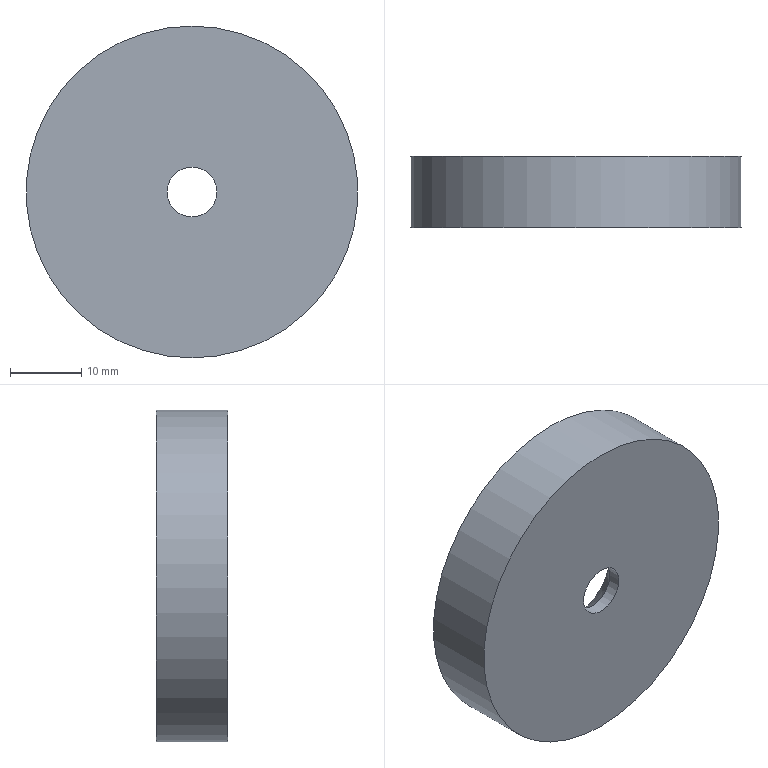Part | STEP file | Lower part of clamping device | 1 solid | 11 faces | box 46.5 x 10 x 46.5 mm | volume 11861 mm3 | plane 5 | cone 3 | cylinder 3 | commonest cylinder face diameters 7 x1 22 x1 46.5 x1
STEP:
#1=CARTESIAN_POINT('',(0.,0.,23.25));
#2=VERTEX_POINT('',#1);
#3=CARTESIAN_POINT('',(0.,0.,0.));
#4=DIRECTION('',(0.,1.,0.));
#5=DIRECTION('',(0.,0.,1.));
#6=AXIS2_PLACEMENT_3D('',#3,#4,#5);
#7=CIRCLE('',#6,23.25);
#8=EDGE_CURVE('',#2,#2,#7,.T.);
#9=ORIENTED_EDGE('',*,*,#8,.F.);
#10=EDGE_LOOP('',(#9));
#11=FACE_BOUND('',#10,.T.);
#12=CARTESIAN_POINT('',(3.5,0.,0.));
#13=VERTEX_POINT('',#12);
#14=CARTESIAN_POINT('',(0.,0.,0.));
#15=DIRECTION('',(0.,1.,0.));
#16=DIRECTION('',(1.,0.,0.));
#17=AXIS2_PLACEMENT_3D('',#14,#15,#16);
#18=CIRCLE('',#17,3.5);
#19=EDGE_CURVE('',#13,#13,#18,.T.);
#20=ORIENTED_EDGE('',*,*,#19,.T.);
#21=EDGE_LOOP('',(#20));
#22=FACE_BOUND('',#21,.T.);
#23=CARTESIAN_POINT('',(0.,0.,0.));
#24=DIRECTION('',(0.,-1.,0.));
#25=DIRECTION('',(0.,0.,1.));
#26=AXIS2_PLACEMENT_3D('',#23,#24,#25);
#27=PLANE('',#26);
#28=ADVANCED_FACE('',(#11,#22),#27,.T.);
#29=CARTESIAN_POINT('',(0.,5.,11.));
#30=VERTEX_POINT('',#29);
#31=CARTESIAN_POINT('',(0.,5.,0.));
#32=DIRECTION('',(0.,1.,0.));
#33=DIRECTION('',(0.,0.,1.));
#34=AXIS2_PLACEMENT_3D('',#31,#32,#33);
#35=CIRCLE('',#34,11.);
#36=EDGE_CURVE('',#30,#30,#35,.T.);
#37=ORIENTED_EDGE('',*,*,#36,.T.);
#38=EDGE_LOOP('',(#37));
#39=FACE_BOUND('',#38,.T.);
#40=CARTESIAN_POINT('',(6.72,5.,0.));
#41=VERTEX_POINT('',#40);
#42=CARTESIAN_POINT('',(0.,5.,0.));
#43=DIRECTION('',(0.,1.,0.));
#44=DIRECTION('',(1.,0.,0.));
#45=AXIS2_PLACEMENT_3D('',#42,#43,#44);
#46=CIRCLE('',#45,6.72);
#47=EDGE_CURVE('',#41,#41,#46,.F.);
#48=ORIENTED_EDGE('',*,*,#47,.T.);
#49=EDGE_LOOP('',(#48));
#50=FACE_BOUND('',#49,.T.);
#51=CARTESIAN_POINT('',(0.,5.,0.));
#52=DIRECTION('',(0.,1.,0.));
#53=DIRECTION('',(0.,0.,1.));
#54=AXIS2_PLACEMENT_3D('',#51,#52,#53);
#55=PLANE('',#54);
#56=ADVANCED_FACE('',(#39,#50),#55,.T.);
#57=ORIENTED_EDGE('',*,*,#47,.F.);
#58=EDGE_LOOP('',(#57));
#59=FACE_OUTER_BOUND('',#58,.T.);
#60=CARTESIAN_POINT('',(3.5,1.78,0.));
#61=VERTEX_POINT('',#60);
#62=CARTESIAN_POINT('',(0.,1.78,0.));
#63=DIRECTION('',(0.,1.,0.));
#64=DIRECTION('',(1.,0.,0.));
#65=AXIS2_PLACEMENT_3D('',#62,#63,#64);
#66=CIRCLE('',#65,3.5);
#67=EDGE_CURVE('',#61,#61,#66,.T.);
#68=ORIENTED_EDGE('',*,*,#67,.F.);
#69=EDGE_LOOP('',(#68));
#70=FACE_OUTER_BOUND('',#69,.T.);
#71=CARTESIAN_POINT('',(0.,3.39,0.));
#72=DIRECTION('',(0.,1.,0.));
#73=DIRECTION('',(1.,0.,0.));
#74=AXIS2_PLACEMENT_3D('',#71,#72,#73);
#75=CONICAL_SURFACE('',#74,5.11,0.7854);
#76=ADVANCED_FACE('',(#59,#70),#75,.F.);
#77=ORIENTED_EDGE('',*,*,#67,.T.);
#78=EDGE_LOOP('',(#77));
#79=FACE_OUTER_BOUND('',#78,.T.);
#80=ORIENTED_EDGE('',*,*,#19,.F.);
#81=EDGE_LOOP('',(#80));
#82=FACE_OUTER_BOUND('',#81,.T.);
#83=CARTESIAN_POINT('',(0.,-35.,0.));
#84=DIRECTION('',(0.,1.,0.));
#85=DIRECTION('',(1.,0.,0.));
#86=AXIS2_PLACEMENT_3D('',#83,#84,#85);
#87=CYLINDRICAL_SURFACE('',#86,3.5);
#88=ADVANCED_FACE('',(#79,#82),#87,.F.);
#89=CARTESIAN_POINT('',(0.,10.,23.25));
#90=VERTEX_POINT('',#89);
#91=CARTESIAN_POINT('',(0.,10.,0.));
#92=DIRECTION('',(0.,1.,0.));
#93=DIRECTION('',(0.,0.,1.));
#94=AXIS2_PLACEMENT_3D('',#91,#92,#93);
#95=CIRCLE('',#94,23.25);
#96=EDGE_CURVE('',#90,#90,#95,.T.);
#97=ORIENTED_EDGE('',*,*,#96,.F.);
#98=EDGE_LOOP('',(#97));
#99=FACE_OUTER_BOUND('',#98,.T.);
#100=ORIENTED_EDGE('',*,*,#8,.T.);
#101=EDGE_LOOP('',(#100));
#102=FACE_OUTER_BOUND('',#101,.T.);
#103=CARTESIAN_POINT('',(0.,0.,0.));
#104=DIRECTION('',(0.,1.,0.));
#105=DIRECTION('',(0.,0.,1.));
#106=AXIS2_PLACEMENT_3D('',#103,#104,#105);
#107=CYLINDRICAL_SURFACE('',#106,23.25);
#108=ADVANCED_FACE('',(#99,#102),#107,.T.);
#109=CARTESIAN_POINT('',(0.,7.5,11.));
#110=VERTEX_POINT('',#109);
#111=CARTESIAN_POINT('',(0.,7.5,0.));
#112=DIRECTION('',(0.,1.,0.));
#113=DIRECTION('',(0.,0.,1.));
#114=AXIS2_PLACEMENT_3D('',#111,#112,#113);
#115=CIRCLE('',#114,11.);
#116=EDGE_CURVE('',#110,#110,#115,.T.);
#117=ORIENTED_EDGE('',*,*,#116,.T.);
#118=EDGE_LOOP('',(#117));
#119=FACE_OUTER_BOUND('',#118,.T.);
#120=ORIENTED_EDGE('',*,*,#36,.F.);
#121=EDGE_LOOP('',(#120));
#122=FACE_OUTER_BOUND('',#121,.T.);
#123=CARTESIAN_POINT('',(0.,7.5,0.));
#124=DIRECTION('',(0.,1.,0.));
#125=DIRECTION('',(0.,0.,1.));
#126=AXIS2_PLACEMENT_3D('',#123,#124,#125);
#127=CYLINDRICAL_SURFACE('',#126,11.);
#128=ADVANCED_FACE('',(#119,#122),#127,.F.);
#129=ORIENTED_EDGE('',*,*,#96,.T.);
#130=EDGE_LOOP('',(#129));
#131=FACE_BOUND('',#130,.T.);
#132=CARTESIAN_POINT('',(0.,10.,22.25));
#133=VERTEX_POINT('',#132);
#134=CARTESIAN_POINT('',(0.,10.,0.));
#135=DIRECTION('',(0.,1.,0.));
#136=DIRECTION('',(0.,0.,1.));
#137=AXIS2_PLACEMENT_3D('',#134,#135,#136);
#138=CIRCLE('',#137,22.25);
#139=EDGE_CURVE('',#133,#133,#138,.T.);
#140=ORIENTED_EDGE('',*,*,#139,.F.);
#141=EDGE_LOOP('',(#140));
#142=FACE_BOUND('',#141,.T.);
#143=CARTESIAN_POINT('',(0.,10.,0.));
#144=DIRECTION('',(0.,1.,0.));
#145=DIRECTION('',(0.,0.,1.));
#146=AXIS2_PLACEMENT_3D('',#143,#144,#145);
#147=PLANE('',#146);
#148=ADVANCED_FACE('',(#131,#142),#147,.T.);
#149=CARTESIAN_POINT('',(0.,7.5,12.));
#150=VERTEX_POINT('',#149);
#151=CARTESIAN_POINT('',(0.,7.5,0.));
#152=DIRECTION('',(0.,1.,0.));
#153=DIRECTION('',(0.,0.,1.));
#154=AXIS2_PLACEMENT_3D('',#151,#152,#153);
#155=CIRCLE('',#154,12.);
#156=EDGE_CURVE('',#150,#150,#155,.T.);
#157=ORIENTED_EDGE('',*,*,#156,.T.);
#158=EDGE_LOOP('',(#157));
#159=FACE_BOUND('',#158,.T.);
#160=ORIENTED_EDGE('',*,*,#116,.F.);
#161=EDGE_LOOP('',(#160));
#162=FACE_BOUND('',#161,.T.);
#163=CARTESIAN_POINT('',(0.,7.5,0.));
#164=DIRECTION('',(0.,1.,0.));
#165=DIRECTION('',(0.,0.,1.));
#166=AXIS2_PLACEMENT_3D('',#163,#164,#165);
#167=PLANE('',#166);
#168=ADVANCED_FACE('',(#159,#162),#167,.T.);
#169=ORIENTED_EDGE('',*,*,#139,.T.);
#170=EDGE_LOOP('',(#169));
#171=FACE_OUTER_BOUND('',#170,.T.);
#172=CARTESIAN_POINT('',(0.,7.,19.25));
#173=VERTEX_POINT('',#172);
#174=CARTESIAN_POINT('',(0.,7.,0.));
#175=DIRECTION('',(0.,1.,0.));
#176=DIRECTION('',(0.,0.,1.));
#177=AXIS2_PLACEMENT_3D('',#174,#175,#176);
#178=CIRCLE('',#177,19.25);
#179=EDGE_CURVE('',#173,#173,#178,.T.);
#180=ORIENTED_EDGE('',*,*,#179,.F.);
#181=EDGE_LOOP('',(#180));
#182=FACE_OUTER_BOUND('',#181,.T.);
#183=CARTESIAN_POINT('',(0.,8.5,0.));
#184=DIRECTION('',(0.,1.,0.));
#185=DIRECTION('',(0.,0.,1.));
#186=AXIS2_PLACEMENT_3D('',#183,#184,#185);
#187=CONICAL_SURFACE('',#186,20.75,0.7854);
#188=ADVANCED_FACE('',(#171,#182),#187,.F.);
#189=ORIENTED_EDGE('',*,*,#156,.F.);
#190=EDGE_LOOP('',(#189));
#191=FACE_OUTER_BOUND('',#190,.T.);
#192=CARTESIAN_POINT('',(0.,7.,12.5));
#193=VERTEX_POINT('',#192);
#194=CARTESIAN_POINT('',(0.,7.,0.));
#195=DIRECTION('',(0.,1.,0.));
#196=DIRECTION('',(0.,0.,1.));
#197=AXIS2_PLACEMENT_3D('',#194,#195,#196);
#198=CIRCLE('',#197,12.5);
#199=EDGE_CURVE('',#193,#193,#198,.T.);
#200=ORIENTED_EDGE('',*,*,#199,.T.);
#201=EDGE_LOOP('',(#200));
#202=FACE_OUTER_BOUND('',#201,.T.);
#203=CARTESIAN_POINT('',(0.,7.25,0.));
#204=DIRECTION('',(0.,-1.,0.));
#205=DIRECTION('',(0.,0.,-1.));
#206=AXIS2_PLACEMENT_3D('',#203,#204,#205);
#207=CONICAL_SURFACE('',#206,12.25,0.7854);
#208=ADVANCED_FACE('',(#191,#202),#207,.T.);
#209=ORIENTED_EDGE('',*,*,#179,.T.);
#210=EDGE_LOOP('',(#209));
#211=FACE_BOUND('',#210,.T.);
#212=ORIENTED_EDGE('',*,*,#199,.F.);
#213=EDGE_LOOP('',(#212));
#214=FACE_BOUND('',#213,.T.);
#215=CARTESIAN_POINT('',(0.,7.,0.));
#216=DIRECTION('',(0.,1.,0.));
#217=DIRECTION('',(0.,0.,1.));
#218=AXIS2_PLACEMENT_3D('',#215,#216,#217);
#219=PLANE('',#218);
#220=ADVANCED_FACE('',(#211,#214),#219,.T.);
#221=CLOSED_SHELL('',(#28,#56,#76,#88,#108,#128,#148,#168,#188,#208,#220));
#222=MANIFOLD_SOLID_BREP('',#221);
#223=(LENGTH_UNIT()NAMED_UNIT(*)SI_UNIT(.MILLI.,.METRE.));
#224=UNCERTAINTY_MEASURE_WITH_UNIT(LENGTH_MEASURE(0.00001),#223,'','');
#225=(NAMED_UNIT(*)PLANE_ANGLE_UNIT()SI_UNIT($,.RADIAN.));
#226=(NAMED_UNIT(*)SI_UNIT($,.STERADIAN.)SOLID_ANGLE_UNIT());
#227=(GEOMETRIC_REPRESENTATION_CONTEXT(3)GLOBAL_UNCERTAINTY_ASSIGNED_CONTEXT((#224))GLOBAL_UNIT_ASSIGNED_CONTEXT((#223,#225,#226))REPRESENTATION_CONTEXT('',''));
#228=ADVANCED_BREP_SHAPE_REPRESENTATION('',(#222),#227);